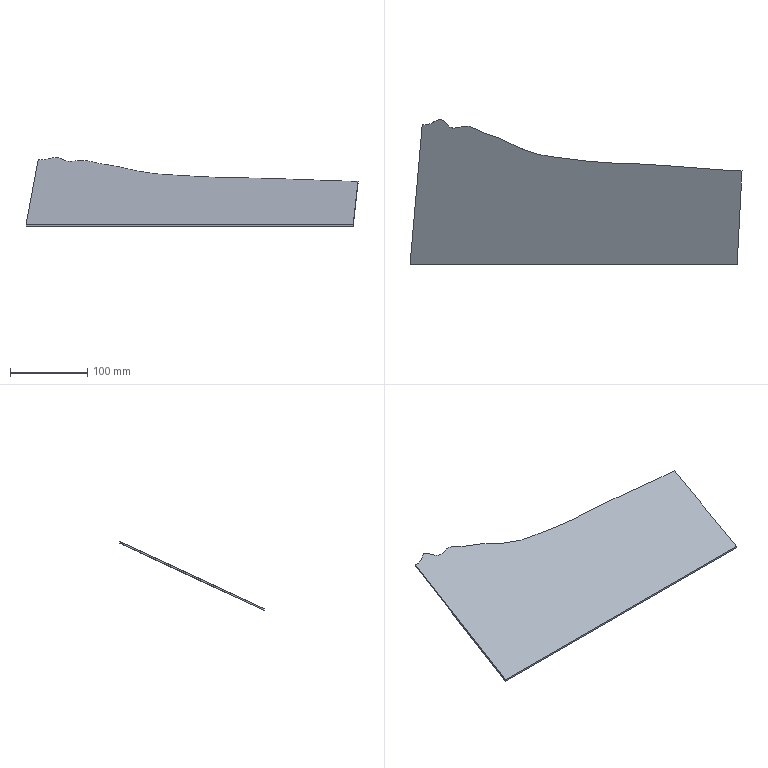Part | NX | features solid 2 | 1 solid | 6 faces | box 430.567 x 187.636 x 89.702 mm | volume 134761 mm3 | plane 5 | spline 1
STEP:
#1=CARTESIAN_POINT('',(-750.357,-485.,-58.495));
#2=VERTEX_POINT('',#1);
#3=CARTESIAN_POINT('',(-326.137,-485.,-58.495));
#4=VERTEX_POINT('',#3);
#5=CARTESIAN_POINT('',(-705.,-485.,-58.495));
#6=DIRECTION('',(-1.,0.,0.));
#7=VECTOR('',#6,1000.);
#8=LINE('',#5,#7);
#9=EDGE_CURVE('',#2,#4,#8,.F.);
#10=ORIENTED_EDGE('',*,*,#9,.T.);
#11=CARTESIAN_POINT('',(-326.137,-485.,-56.288));
#12=VERTEX_POINT('',#11);
#13=CARTESIAN_POINT('',(-326.137,-485.,-75.));
#14=DIRECTION('',(0.,0.,-1.));
#15=VECTOR('',#14,1000.);
#16=LINE('',#13,#15);
#17=EDGE_CURVE('',#4,#12,#16,.F.);
#18=ORIENTED_EDGE('',*,*,#17,.T.);
#19=CARTESIAN_POINT('',(-750.357,-485.,-56.288));
#20=VERTEX_POINT('',#19);
#21=CARTESIAN_POINT('',(-705.,-485.,-56.288));
#22=DIRECTION('',(-1.,0.,0.));
#23=VECTOR('',#22,1000.);
#24=LINE('',#21,#23);
#25=EDGE_CURVE('',#20,#12,#24,.F.);
#26=ORIENTED_EDGE('',*,*,#25,.F.);
#27=CARTESIAN_POINT('',(-750.357,-485.,-187.478));
#28=DIRECTION('',(0.,0.,-1.));
#29=VECTOR('',#28,1000.);
#30=LINE('',#27,#29);
#31=EDGE_CURVE('',#2,#20,#30,.F.);
#32=ORIENTED_EDGE('',*,*,#31,.F.);
#33=EDGE_LOOP('',(#10,#18,#26,#32));
#34=FACE_BOUND('',#33,.T.);
#35=CARTESIAN_POINT('',(691.22,-485.,-75.));
#36=DIRECTION('',(0.,1.,0.));
#37=DIRECTION('',(-1.,0.,0.));
#38=AXIS2_PLACEMENT_3D('',#35,#36,#37);
#39=PLANE('',#38);
#40=ADVANCED_FACE('',(#34),#39,.F.);
#41=ORIENTED_EDGE('',*,*,#25,.T.);
#42=CARTESIAN_POINT('',(-319.79,-363.898,0.1825));
#43=VERTEX_POINT('',#42);
#44=CARTESIAN_POINT('',(-348.889,-919.115,-258.72));
#45=DIRECTION('',(0.04745,0.9053,0.4221));
#46=VECTOR('',#45,1000.);
#47=LINE('',#44,#46);
#48=EDGE_CURVE('',#12,#43,#47,.T.);
#49=ORIENTED_EDGE('',*,*,#48,.T.);
#50=CARTESIAN_POINT('',(-734.467,-303.374,28.405));
#51=VERTEX_POINT('',#50);
#52=CARTESIAN_POINT('',(-734.467,-303.374,28.405));
#53=CARTESIAN_POINT('',(-733.483,-303.791,28.211));
#54=CARTESIAN_POINT('',(-731.322,-304.207,28.016));
#55=CARTESIAN_POINT('',(-726.97,-303.884,28.167));
#56=CARTESIAN_POINT('',(-722.915,-302.399,28.86));
#57=CARTESIAN_POINT('',(-719.18,-300.436,29.775));
#58=CARTESIAN_POINT('',(-716.424,-298.859,30.511));
#59=CARTESIAN_POINT('',(-714.032,-297.743,31.031));
#60=CARTESIAN_POINT('',(-711.853,-297.288,31.243));
#61=CARTESIAN_POINT('',(-709.609,-297.51,31.14));
#62=CARTESIAN_POINT('',(-707.245,-298.919,30.482));
#63=CARTESIAN_POINT('',(-705.048,-301.189,29.424));
#64=CARTESIAN_POINT('',(-702.907,-303.512,28.341));
#65=CARTESIAN_POINT('',(-700.657,-305.722,27.31));
#66=CARTESIAN_POINT('',(-697.931,-307.574,26.447));
#67=CARTESIAN_POINT('',(-694.669,-308.54,25.996));
#68=CARTESIAN_POINT('',(-691.259,-308.363,26.079));
#69=CARTESIAN_POINT('',(-686.916,-307.429,26.514));
#70=CARTESIAN_POINT('',(-681.523,-305.954,27.202));
#71=CARTESIAN_POINT('',(-674.787,-305.859,27.247));
#72=CARTESIAN_POINT('',(-668.45,-307.874,26.307));
#73=CARTESIAN_POINT('',(-662.621,-310.834,24.927));
#74=CARTESIAN_POINT('',(-656.8,-313.853,23.519));
#75=CARTESIAN_POINT('',(-648.637,-317.026,22.039));
#76=CARTESIAN_POINT('',(-640.008,-319.241,21.006));
#77=CARTESIAN_POINT('',(-631.871,-322.465,19.503));
#78=CARTESIAN_POINT('',(-624.049,-326.383,17.676));
#79=CARTESIAN_POINT('',(-614.457,-331.791,15.154));
#80=CARTESIAN_POINT('',(-604.338,-335.841,13.265));
#81=CARTESIAN_POINT('',(-596.12,-338.772,11.899));
#82=CARTESIAN_POINT('',(-589.907,-340.843,10.933));
#83=CARTESIAN_POINT('',(-583.578,-342.62,10.104));
#84=CARTESIAN_POINT('',(-574.918,-344.424,9.263));
#85=CARTESIAN_POINT('',(-563.773,-345.873,8.588));
#86=CARTESIAN_POINT('',(-550.254,-347.192,7.972));
#87=CARTESIAN_POINT('',(-536.793,-348.851,7.199));
#88=CARTESIAN_POINT('',(-523.384,-350.97,6.211));
#89=CARTESIAN_POINT('',(-509.923,-352.661,5.422));
#90=CARTESIAN_POINT('',(-496.341,-353.362,5.095));
#91=CARTESIAN_POINT('',(-478.191,-353.962,4.816));
#92=CARTESIAN_POINT('',(-455.493,-354.6,4.518));
#93=CARTESIAN_POINT('',(-428.324,-356.232,3.757));
#94=CARTESIAN_POINT('',(-401.19,-358.312,2.787));
#95=CARTESIAN_POINT('',(-378.582,-360.103,1.952));
#96=CARTESIAN_POINT('',(-360.475,-361.266,1.41));
#97=CARTESIAN_POINT('',(-346.918,-362.419,0.8721));
#98=CARTESIAN_POINT('',(-333.358,-363.644,0.301));
#99=CARTESIAN_POINT('',(-324.313,-363.87,0.1954));
#100=CARTESIAN_POINT('',(-319.79,-363.898,0.1825));
#101=B_SPLINE_CURVE_WITH_KNOTS('',3,(#52,#53,#54,#55,#56,#57,#58,#59,#60,#61,#62,#63,#64,#65,#66,#67,#68,#69,#70,#71,#72,#73,#74,#75,#76,#77,#78,#79,#80,#81,#82,#83,#84,#85,#86,#87,#88,#89,#90,#91,#92,#93,#94,#95,#96,#97,#98,#99,#100),.UNSPECIFIED.,.F.,.F.,(4,1,1,1,1,1,1,1,1,1,1,1,1,1,1,1,1,1,1,1,1,1,1,1,1,1,1,1,1,1,1,1,1,1,1,1,1,1,1,1,1,1,1,1,1,1,4),(0.04087,0.04411,0.04734,0.05382,0.05706,0.0603,0.06354,0.06516,0.06678,0.07002,0.07326,0.07649,0.07973,0.08297,0.08621,0.08945,0.09269,0.09917,0.1056,0.1121,0.1186,0.1251,0.1316,0.1445,0.151,0.1575,0.1704,0.1834,0.1899,0.1963,0.2028,0.2093,0.2222,0.2352,0.2482,0.2611,0.2741,0.287,0.3,0.3259,0.3518,0.3777,0.4036,0.4166,0.4295,0.4425,0.4554),.UNSPECIFIED.);
#102=EDGE_CURVE('',#51,#43,#101,.T.);
#103=ORIENTED_EDGE('',*,*,#102,.F.);
#104=CARTESIAN_POINT('',(-754.694,-534.576,-79.406));
#105=DIRECTION('',(0.07904,0.9035,0.4213));
#106=VECTOR('',#105,1000.);
#107=LINE('',#104,#106);
#108=EDGE_CURVE('',#20,#51,#107,.T.);
#109=ORIENTED_EDGE('',*,*,#108,.F.);
#110=EDGE_LOOP('',(#41,#49,#103,#109));
#111=FACE_BOUND('',#110,.T.);
#112=CARTESIAN_POINT('',(-705.,-903.785,-251.571));
#113=DIRECTION('',(0.,-0.4226,0.9063));
#114=DIRECTION('',(1.,0.,0.));
#115=AXIS2_PLACEMENT_3D('',#112,#113,#114);
#116=PLANE('',#115);
#117=ADVANCED_FACE('',(#111),#116,.T.);
#118=CARTESIAN_POINT('',(-319.79,-363.898,-2.024));
#119=VERTEX_POINT('',#118);
#120=CARTESIAN_POINT('',(-348.845,-918.272,-260.533));
#121=DIRECTION('',(0.04745,0.9053,0.4221));
#122=VECTOR('',#121,1000.);
#123=LINE('',#120,#122);
#124=EDGE_CURVE('',#4,#119,#123,.T.);
#125=ORIENTED_EDGE('',*,*,#124,.F.);
#126=ORIENTED_EDGE('',*,*,#9,.F.);
#127=CARTESIAN_POINT('',(-734.467,-303.374,26.198));
#128=VERTEX_POINT('',#127);
#129=CARTESIAN_POINT('',(-754.621,-533.736,-81.221));
#130=DIRECTION('',(0.07904,0.9035,0.4213));
#131=VECTOR('',#130,1000.);
#132=LINE('',#129,#131);
#133=EDGE_CURVE('',#2,#128,#132,.T.);
#134=ORIENTED_EDGE('',*,*,#133,.T.);
#135=CARTESIAN_POINT('',(-734.467,-303.374,26.198));
#136=CARTESIAN_POINT('',(-732.558,-304.183,25.821));
#137=CARTESIAN_POINT('',(-728.217,-304.263,25.784));
#138=CARTESIAN_POINT('',(-723.354,-302.586,26.566));
#139=CARTESIAN_POINT('',(-719.722,-300.734,27.429));
#140=CARTESIAN_POINT('',(-717.066,-299.227,28.132));
#141=CARTESIAN_POINT('',(-714.389,-297.852,28.773));
#142=CARTESIAN_POINT('',(-711.252,-297.048,29.148));
#143=CARTESIAN_POINT('',(-708.157,-298.187,28.617));
#144=CARTESIAN_POINT('',(-705.938,-300.248,27.656));
#145=CARTESIAN_POINT('',(-703.87,-302.463,26.623));
#146=CARTESIAN_POINT('',(-701.787,-304.669,25.595));
#147=CARTESIAN_POINT('',(-699.476,-306.626,24.682));
#148=CARTESIAN_POINT('',(-696.565,-308.142,23.975));
#149=CARTESIAN_POINT('',(-693.211,-308.563,23.779));
#150=CARTESIAN_POINT('',(-688.829,-307.965,24.058));
#151=CARTESIAN_POINT('',(-684.559,-306.704,24.646));
#152=CARTESIAN_POINT('',(-680.185,-306.006,24.971));
#153=CARTESIAN_POINT('',(-675.652,-305.891,25.024));
#154=CARTESIAN_POINT('',(-670.258,-307.12,24.452));
#155=CARTESIAN_POINT('',(-664.254,-309.951,23.131));
#156=CARTESIAN_POINT('',(-658.482,-313.044,21.689));
#157=CARTESIAN_POINT('',(-650.371,-316.51,20.073));
#158=CARTESIAN_POINT('',(-641.691,-318.741,19.032));
#159=CARTESIAN_POINT('',(-633.394,-321.796,17.608));
#160=CARTESIAN_POINT('',(-625.448,-325.597,15.836));
#161=CARTESIAN_POINT('',(-617.766,-329.972,13.796));
#162=CARTESIAN_POINT('',(-609.783,-333.669,12.071));
#163=CARTESIAN_POINT('',(-603.635,-336.077,10.949));
#164=CARTESIAN_POINT('',(-597.412,-338.316,9.905));
#165=CARTESIAN_POINT('',(-591.145,-340.453,8.908));
#166=CARTESIAN_POINT('',(-584.761,-342.324,8.036));
#167=CARTESIAN_POINT('',(-575.995,-344.257,7.134));
#168=CARTESIAN_POINT('',(-564.694,-345.777,6.426));
#169=CARTESIAN_POINT('',(-551.153,-347.101,5.808));
#170=CARTESIAN_POINT('',(-537.626,-348.731,5.048));
#171=CARTESIAN_POINT('',(-524.16,-350.846,4.062));
#172=CARTESIAN_POINT('',(-510.651,-352.602,3.243));
#173=CARTESIAN_POINT('',(-497.028,-353.337,2.9));
#174=CARTESIAN_POINT('',(-478.821,-353.945,2.617));
#175=CARTESIAN_POINT('',(-456.052,-354.575,2.323));
#176=CARTESIAN_POINT('',(-428.786,-356.198,1.566));
#177=CARTESIAN_POINT('',(-401.547,-358.283,0.5937));
#178=CARTESIAN_POINT('',(-378.851,-360.084,-0.2461));
#179=CARTESIAN_POINT('',(-360.678,-361.252,-0.7907));
#180=CARTESIAN_POINT('',(-347.065,-362.404,-1.328));
#181=CARTESIAN_POINT('',(-333.457,-363.639,-1.904));
#182=CARTESIAN_POINT('',(-324.349,-363.87,-2.011));
#183=CARTESIAN_POINT('',(-319.79,-363.898,-2.024));
#184=B_SPLINE_CURVE_WITH_KNOTS('',3,(#135,#136,#137,#138,#139,#140,#141,#142,#143,#144,#145,#146,#147,#148,#149,#150,#151,#152,#153,#154,#155,#156,#157,#158,#159,#160,#161,#162,#163,#164,#165,#166,#167,#168,#169,#170,#171,#172,#173,#174,#175,#176,#177,#178,#179,#180,#181,#182,#183),.UNSPECIFIED.,.F.,.F.,(4,1,1,1,1,1,1,1,1,1,1,1,1,1,1,1,1,1,1,1,1,1,1,1,1,1,1,1,1,1,1,1,1,1,1,1,1,1,1,1,1,1,1,1,1,1,4),(0.04208,0.04827,0.05447,0.05756,0.06066,0.06375,0.06685,0.06994,0.07304,0.07613,0.07923,0.08232,0.08542,0.08851,0.09161,0.0978,0.1009,0.104,0.1102,0.1164,0.1226,0.1288,0.1411,0.1473,0.1535,0.1659,0.1721,0.1783,0.1845,0.1907,0.1968,0.203,0.2154,0.2278,0.2402,0.2526,0.2649,0.2773,0.2897,0.3145,0.3392,0.364,0.3888,0.4011,0.4135,0.4259,0.4383),.UNSPECIFIED.);
#185=EDGE_CURVE('',#128,#119,#184,.T.);
#186=ORIENTED_EDGE('',*,*,#185,.T.);
#187=EDGE_LOOP('',(#125,#126,#134,#186));
#188=FACE_BOUND('',#187,.T.);
#189=CARTESIAN_POINT('',(-705.,-902.939,-253.384));
#190=DIRECTION('',(0.,-0.4226,0.9063));
#191=DIRECTION('',(1.,0.,0.));
#192=AXIS2_PLACEMENT_3D('',#189,#190,#191);
#193=PLANE('',#192);
#194=ADVANCED_FACE('',(#188),#193,.F.);
#195=CARTESIAN_POINT('',(-319.79,-363.898,-1.028));
#196=DIRECTION('',(0.,0.,-1.));
#197=VECTOR('',#196,1000.);
#198=LINE('',#195,#197);
#199=EDGE_CURVE('',#119,#43,#198,.F.);
#200=ORIENTED_EDGE('',*,*,#199,.F.);
#201=ORIENTED_EDGE('',*,*,#185,.F.);
#202=CARTESIAN_POINT('',(-734.467,-303.374,600.));
#203=DIRECTION('',(0.,0.,-1.));
#204=VECTOR('',#203,1000.);
#205=LINE('',#202,#204);
#206=EDGE_CURVE('',#128,#51,#205,.F.);
#207=ORIENTED_EDGE('',*,*,#206,.T.);
#208=ORIENTED_EDGE('',*,*,#102,.T.);
#209=EDGE_LOOP('',(#200,#201,#207,#208));
#210=FACE_BOUND('',#209,.T.);
#211=CARTESIAN_POINT('',(-319.79,-363.898,31.422));
#212=CARTESIAN_POINT('',(-319.79,-363.898,-2.224));
#213=CARTESIAN_POINT('',(-324.254,-363.87,31.422));
#214=CARTESIAN_POINT('',(-324.254,-363.87,-2.224));
#215=CARTESIAN_POINT('',(-333.182,-363.65,31.422));
#216=CARTESIAN_POINT('',(-333.182,-363.65,-2.224));
#217=CARTESIAN_POINT('',(-346.524,-362.459,31.422));
#218=CARTESIAN_POINT('',(-346.524,-362.459,-2.224));
#219=CARTESIAN_POINT('',(-359.865,-361.308,31.422));
#220=CARTESIAN_POINT('',(-359.865,-361.308,-2.224));
#221=CARTESIAN_POINT('',(-377.685,-360.165,31.422));
#222=CARTESIAN_POINT('',(-377.685,-360.165,-2.224));
#223=CARTESIAN_POINT('',(-399.934,-358.415,31.422));
#224=CARTESIAN_POINT('',(-399.934,-358.415,-2.224));
#225=CARTESIAN_POINT('',(-426.638,-356.354,31.422));
#226=CARTESIAN_POINT('',(-426.638,-356.354,-2.224));
#227=CARTESIAN_POINT('',(-453.373,-354.703,31.422));
#228=CARTESIAN_POINT('',(-453.373,-354.703,-2.224));
#229=CARTESIAN_POINT('',(-475.682,-354.026,31.422));
#230=CARTESIAN_POINT('',(-475.682,-354.026,-2.224));
#231=CARTESIAN_POINT('',(-493.527,-353.463,31.422));
#232=CARTESIAN_POINT('',(-493.527,-353.463,-2.224));
#233=CARTESIAN_POINT('',(-506.913,-352.873,31.422));
#234=CARTESIAN_POINT('',(-506.913,-352.873,-2.224));
#235=CARTESIAN_POINT('',(-520.228,-351.456,31.422));
#236=CARTESIAN_POINT('',(-520.228,-351.456,-2.224));
#237=CARTESIAN_POINT('',(-533.458,-349.348,31.422));
#238=CARTESIAN_POINT('',(-533.458,-349.348,-2.224));
#239=CARTESIAN_POINT('',(-546.733,-347.575,31.422));
#240=CARTESIAN_POINT('',(-546.733,-347.575,-2.224));
#241=CARTESIAN_POINT('',(-560.049,-346.24,31.422));
#242=CARTESIAN_POINT('',(-560.049,-346.24,-2.224));
#243=CARTESIAN_POINT('',(-573.381,-344.732,31.422));
#244=CARTESIAN_POINT('',(-573.381,-344.732,-2.224));
#245=CARTESIAN_POINT('',(-586.508,-342.086,31.422));
#246=CARTESIAN_POINT('',(-586.508,-342.086,-2.224));
#247=CARTESIAN_POINT('',(-599.197,-337.722,31.422));
#248=CARTESIAN_POINT('',(-599.197,-337.722,-2.224));
#249=CARTESIAN_POINT('',(-609.658,-333.828,31.422));
#250=CARTESIAN_POINT('',(-609.658,-333.828,-2.224));
#251=CARTESIAN_POINT('',(-617.688,-329.911,31.422));
#252=CARTESIAN_POINT('',(-617.688,-329.911,-2.224));
#253=CARTESIAN_POINT('',(-623.58,-326.714,31.422));
#254=CARTESIAN_POINT('',(-623.58,-326.714,-2.224));
#255=CARTESIAN_POINT('',(-629.499,-323.587,31.422));
#256=CARTESIAN_POINT('',(-629.499,-323.587,-2.224));
#257=CARTESIAN_POINT('',(-635.627,-320.901,31.422));
#258=CARTESIAN_POINT('',(-635.627,-320.901,-2.224));
#259=CARTESIAN_POINT('',(-641.988,-318.774,31.422));
#260=CARTESIAN_POINT('',(-641.988,-318.774,-2.224));
#261=CARTESIAN_POINT('',(-648.429,-316.955,31.422));
#262=CARTESIAN_POINT('',(-648.429,-316.955,-2.224));
#263=CARTESIAN_POINT('',(-654.761,-314.735,31.422));
#264=CARTESIAN_POINT('',(-654.761,-314.735,-2.224));
#265=CARTESIAN_POINT('',(-660.784,-311.838,31.422));
#266=CARTESIAN_POINT('',(-660.784,-311.838,-2.224));
#267=CARTESIAN_POINT('',(-666.714,-308.684,31.422));
#268=CARTESIAN_POINT('',(-666.714,-308.684,-2.224));
#269=CARTESIAN_POINT('',(-672.976,-306.228,31.422));
#270=CARTESIAN_POINT('',(-672.976,-306.228,-2.224));
#271=CARTESIAN_POINT('',(-679.738,-305.707,31.422));
#272=CARTESIAN_POINT('',(-679.738,-305.707,-2.224));
#273=CARTESIAN_POINT('',(-685.214,-306.94,31.422));
#274=CARTESIAN_POINT('',(-685.214,-306.94,-2.224));
#275=CARTESIAN_POINT('',(-689.528,-308.036,31.422));
#276=CARTESIAN_POINT('',(-689.528,-308.036,-2.224));
#277=CARTESIAN_POINT('',(-692.873,-308.544,31.422));
#278=CARTESIAN_POINT('',(-692.873,-308.544,-2.224));
#279=CARTESIAN_POINT('',(-696.224,-308.25,31.422));
#280=CARTESIAN_POINT('',(-696.224,-308.25,-2.224));
#281=CARTESIAN_POINT('',(-699.298,-306.772,31.422));
#282=CARTESIAN_POINT('',(-699.298,-306.772,-2.224));
#283=CARTESIAN_POINT('',(-701.842,-304.631,31.422));
#284=CARTESIAN_POINT('',(-701.842,-304.631,-2.224));
#285=CARTESIAN_POINT('',(-704.128,-302.185,31.422));
#286=CARTESIAN_POINT('',(-704.128,-302.185,-2.224));
#287=CARTESIAN_POINT('',(-706.442,-299.699,31.422));
#288=CARTESIAN_POINT('',(-706.442,-299.699,-2.224));
#289=CARTESIAN_POINT('',(-709.088,-297.574,31.422));
#290=CARTESIAN_POINT('',(-709.088,-297.574,-2.224));
#291=CARTESIAN_POINT('',(-712.539,-297.156,31.422));
#292=CARTESIAN_POINT('',(-712.539,-297.156,-2.224));
#293=CARTESIAN_POINT('',(-715.687,-298.464,31.422));
#294=CARTESIAN_POINT('',(-715.687,-298.464,-2.224));
#295=CARTESIAN_POINT('',(-718.598,-300.106,31.422));
#296=CARTESIAN_POINT('',(-718.598,-300.106,-2.224));
#297=CARTESIAN_POINT('',(-722.519,-302.229,31.422));
#298=CARTESIAN_POINT('',(-722.519,-302.229,-2.224));
#299=CARTESIAN_POINT('',(-726.742,-303.843,31.422));
#300=CARTESIAN_POINT('',(-726.742,-303.843,-2.224));
#301=CARTESIAN_POINT('',(-731.212,-304.217,31.422));
#302=CARTESIAN_POINT('',(-731.212,-304.217,-2.224));
#303=CARTESIAN_POINT('',(-733.436,-303.811,31.422));
#304=CARTESIAN_POINT('',(-733.436,-303.811,-2.224));
#305=CARTESIAN_POINT('',(-734.467,-303.374,31.422));
#306=CARTESIAN_POINT('',(-734.467,-303.374,-2.224));
#307=B_SPLINE_SURFACE_WITH_KNOTS('',3,1,((#211,#212),(#213,#214),(#215,#216),(#217,#218),(#219,#220),(#221,#222),(#223,#224),(#225,#226),(#227,#228),(#229,#230),(#231,#232),(#233,#234),(#235,#236),(#237,#238),(#239,#240),(#241,#242),(#243,#244),(#245,#246),(#247,#248),(#249,#250),(#251,#252),(#253,#254),(#255,#256),(#257,#258),(#259,#260),(#261,#262),(#263,#264),(#265,#266),(#267,#268),(#269,#270),(#271,#272),(#273,#274),(#275,#276),(#277,#278),(#279,#280),(#281,#282),(#283,#284),(#285,#286),(#287,#288),(#289,#290),(#291,#292),(#293,#294),(#295,#296),(#297,#298),(#299,#300),(#301,#302),(#303,#304),(#305,#306)),.SURF_OF_LINEAR_EXTRUSION.,.F.,.F.,.F.,(4,1,1,1,1,1,1,1,1,1,1,1,1,1,1,1,1,1,1,1,1,1,1,1,1,1,1,1,1,1,1,1,1,1,1,1,1,1,1,1,1,1,1,1,1,4),(2,2),(0.2881,0.2911,0.294,0.297,0.2999,0.3058,0.3117,0.3176,0.3235,0.3264,0.3294,0.3323,0.3353,0.3382,0.3412,0.3441,0.347,0.35,0.3529,0.3544,0.3559,0.3574,0.3588,0.3603,0.3618,0.3632,0.3647,0.3662,0.3677,0.3691,0.3706,0.3713,0.3721,0.3728,0.3736,0.3743,0.375,0.3758,0.3765,0.3772,0.378,0.3787,0.3794,0.3809,0.3816,0.3824),(0.,1.),.UNSPECIFIED.);
#308=ADVANCED_FACE('',(#210),#307,.F.);
#309=ORIENTED_EDGE('',*,*,#206,.F.);
#310=ORIENTED_EDGE('',*,*,#133,.F.);
#311=ORIENTED_EDGE('',*,*,#31,.T.);
#312=ORIENTED_EDGE('',*,*,#108,.T.);
#313=EDGE_LOOP('',(#309,#310,#311,#312));
#314=FACE_BOUND('',#313,.T.);
#315=CARTESIAN_POINT('',(-750.319,-484.564,-187.478));
#316=DIRECTION('',(-0.9962,0.08716,0.));
#317=DIRECTION('',(-0.08716,-0.9962,0.));
#318=AXIS2_PLACEMENT_3D('',#315,#316,#317);
#319=PLANE('',#318);
#320=ADVANCED_FACE('',(#314),#319,.T.);
#321=ORIENTED_EDGE('',*,*,#17,.F.);
#322=ORIENTED_EDGE('',*,*,#124,.T.);
#323=ORIENTED_EDGE('',*,*,#199,.T.);
#324=ORIENTED_EDGE('',*,*,#48,.F.);
#325=EDGE_LOOP('',(#321,#322,#323,#324));
#326=FACE_BOUND('',#325,.T.);
#327=CARTESIAN_POINT('',(-324.897,-461.336,-85.));
#328=DIRECTION('',(0.9986,-0.05234,0.));
#329=DIRECTION('',(0.05234,0.9986,0.));
#330=AXIS2_PLACEMENT_3D('',#327,#328,#329);
#331=PLANE('',#330);
#332=ADVANCED_FACE('',(#326),#331,.T.);
#333=CLOSED_SHELL('',(#40,#117,#194,#308,#320,#332));
#334=MANIFOLD_SOLID_BREP('',#333);
#335=(LENGTH_UNIT()NAMED_UNIT(*)SI_UNIT(.MILLI.,.METRE.));
#336=UNCERTAINTY_MEASURE_WITH_UNIT(LENGTH_MEASURE(0.0508),#335,'','');
#337=(NAMED_UNIT(*)PLANE_ANGLE_UNIT()SI_UNIT($,.RADIAN.));
#338=(NAMED_UNIT(*)SI_UNIT($,.STERADIAN.)SOLID_ANGLE_UNIT());
#339=(GEOMETRIC_REPRESENTATION_CONTEXT(3)GLOBAL_UNCERTAINTY_ASSIGNED_CONTEXT((#336))GLOBAL_UNIT_ASSIGNED_CONTEXT((#335,#337,#338))REPRESENTATION_CONTEXT('',''));
#340=ADVANCED_BREP_SHAPE_REPRESENTATION('',(#334),#339);